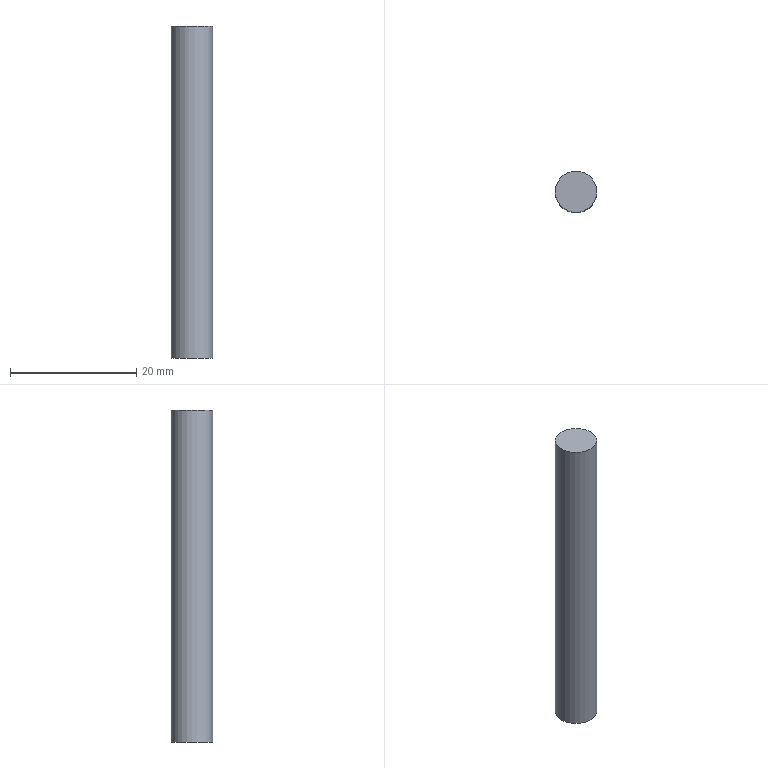Part | STEP file | lll_id134_x_t | 1 solid | 3 faces | box 6.56 x 6.56 x 52.5 mm | volume 1774 mm3 | plane 2 | cylinder 1 | commonest cylinder face diameters 6.56 x1
STEP:
#1=CARTESIAN_POINT('',(200.053,-30.,52.5));
#2=VERTEX_POINT('',#1);
#3=CARTESIAN_POINT('',(196.773,-30.,52.5));
#4=DIRECTION('',(0.,0.,-1.));
#5=DIRECTION('',(1.,0.,0.));
#6=AXIS2_PLACEMENT_3D('',#3,#4,#5);
#7=CIRCLE('',#6,3.28);
#8=EDGE_CURVE('',#2,#2,#7,.T.);
#9=ORIENTED_EDGE('',*,*,#8,.F.);
#10=EDGE_LOOP('',(#9));
#11=FACE_OUTER_BOUND('',#10,.T.);
#12=CARTESIAN_POINT('',(196.773,-30.,52.5));
#13=DIRECTION('',(0.,0.,1.));
#14=DIRECTION('',(1.,0.,0.));
#15=AXIS2_PLACEMENT_3D('',#12,#13,#14);
#16=PLANE('',#15);
#17=ADVANCED_FACE('',(#11),#16,.T.);
#18=CARTESIAN_POINT('',(200.053,-30.,0.00002405));
#19=VERTEX_POINT('',#18);
#20=CARTESIAN_POINT('',(196.773,-30.,0.00002405));
#21=DIRECTION('',(0.,0.,1.));
#22=DIRECTION('',(1.,0.,0.));
#23=AXIS2_PLACEMENT_3D('',#20,#21,#22);
#24=CIRCLE('',#23,3.28);
#25=EDGE_CURVE('',#19,#19,#24,.T.);
#26=ORIENTED_EDGE('',*,*,#25,.F.);
#27=EDGE_LOOP('',(#26));
#28=FACE_OUTER_BOUND('',#27,.T.);
#29=CARTESIAN_POINT('',(196.773,-30.,0.00002405));
#30=DIRECTION('',(0.,0.,-1.));
#31=DIRECTION('',(-1.,0.,0.));
#32=AXIS2_PLACEMENT_3D('',#29,#30,#31);
#33=PLANE('',#32);
#34=ADVANCED_FACE('',(#28),#33,.T.);
#35=ORIENTED_EDGE('',*,*,#8,.T.);
#36=EDGE_LOOP('',(#35));
#37=FACE_BOUND('',#36,.T.);
#38=ORIENTED_EDGE('',*,*,#25,.T.);
#39=EDGE_LOOP('',(#38));
#40=FACE_BOUND('',#39,.T.);
#41=CARTESIAN_POINT('',(196.773,-30.,0.00002405));
#42=DIRECTION('',(0.,0.,1.));
#43=DIRECTION('',(1.,0.,0.));
#44=AXIS2_PLACEMENT_3D('',#41,#42,#43);
#45=CYLINDRICAL_SURFACE('',#44,3.28);
#46=ADVANCED_FACE('',(#37,#40),#45,.T.);
#47=CLOSED_SHELL('',(#17,#34,#46));
#48=MANIFOLD_SOLID_BREP('',#47);
#49=(LENGTH_UNIT()NAMED_UNIT(*)SI_UNIT(.MILLI.,.METRE.));
#50=UNCERTAINTY_MEASURE_WITH_UNIT(LENGTH_MEASURE(0.00002),#49,'','');
#51=(NAMED_UNIT(*)PLANE_ANGLE_UNIT()SI_UNIT($,.RADIAN.));
#52=PLANE_ANGLE_MEASURE_WITH_UNIT(PLANE_ANGLE_MEASURE(0.01745),#51);
#53=DIMENSIONAL_EXPONENTS(0.,0.,0.,0.,0.,0.,0.);
#54=(CONVERSION_BASED_UNIT('DEGREE',#52)NAMED_UNIT(#53)PLANE_ANGLE_UNIT());
#55=(NAMED_UNIT(*)SI_UNIT($,.STERADIAN.)SOLID_ANGLE_UNIT());
#56=(GEOMETRIC_REPRESENTATION_CONTEXT(3)GLOBAL_UNCERTAINTY_ASSIGNED_CONTEXT((#50))GLOBAL_UNIT_ASSIGNED_CONTEXT((#49,#54,#55))REPRESENTATION_CONTEXT('',''));
#57=ADVANCED_BREP_SHAPE_REPRESENTATION('',(#48),#56);